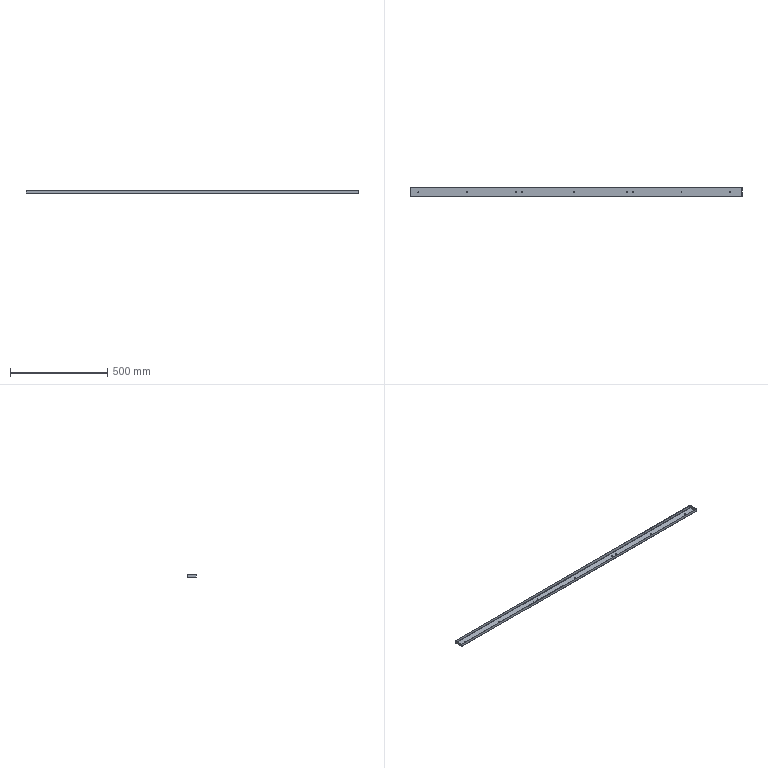Part | STEP file | [01]-3 | 1 solid | 35 faces | box 1704 x 46 x 15 mm | volume 124954 mm3 | cylinder 22 | plane 13 | commonest cylinder face diameters 5 x18 2 x2 4 x2
STEP:
#1=CARTESIAN_POINT('',(1641.,23.,1.));
#2=VERTEX_POINT('',#1);
#3=CARTESIAN_POINT('',(1646.,23.,1.));
#4=VERTEX_POINT('',#3);
#5=CARTESIAN_POINT('',(1643.5,23.,1.));
#6=DIRECTION('',(0.,0.,-1.));
#7=DIRECTION('',(1.,0.,0.));
#8=AXIS2_PLACEMENT_3D('',#5,#6,#7);
#9=CIRCLE('',#8,2.5);
#10=EDGE_CURVE('',#2,#4,#9,.T.);
#11=ORIENTED_EDGE('',*,*,#10,.F.);
#12=CARTESIAN_POINT('',(1641.,23.,0.));
#13=VERTEX_POINT('',#12);
#14=CARTESIAN_POINT('',(1641.,23.,1.));
#15=DIRECTION('',(0.,0.,-1.));
#16=VECTOR('',#15,1000.);
#17=LINE('',#14,#16);
#18=EDGE_CURVE('',#2,#13,#17,.T.);
#19=ORIENTED_EDGE('',*,*,#18,.T.);
#20=CARTESIAN_POINT('',(1646.,23.,0.));
#21=VERTEX_POINT('',#20);
#22=CARTESIAN_POINT('',(1643.5,23.,0.));
#23=DIRECTION('',(0.,0.,1.));
#24=DIRECTION('',(-1.,0.,0.));
#25=AXIS2_PLACEMENT_3D('',#22,#23,#24);
#26=CIRCLE('',#25,2.5);
#27=EDGE_CURVE('',#21,#13,#26,.T.);
#28=ORIENTED_EDGE('',*,*,#27,.F.);
#29=CARTESIAN_POINT('',(1646.,23.,1.));
#30=DIRECTION('',(0.,0.,-1.));
#31=VECTOR('',#30,1000.);
#32=LINE('',#29,#31);
#33=EDGE_CURVE('',#4,#21,#32,.T.);
#34=ORIENTED_EDGE('',*,*,#33,.F.);
#35=EDGE_LOOP('',(#11,#19,#28,#34));
#36=FACE_OUTER_BOUND('',#35,.T.);
#37=CARTESIAN_POINT('',(1643.5,23.,1.));
#38=DIRECTION('',(0.,0.,-1.));
#39=DIRECTION('',(1.,0.,0.));
#40=AXIS2_PLACEMENT_3D('',#37,#38,#39);
#41=CYLINDRICAL_SURFACE('',#40,2.5);
#42=ADVANCED_FACE('',(#36),#41,.F.);
#43=CARTESIAN_POINT('',(1391.,23.,1.));
#44=VERTEX_POINT('',#43);
#45=CARTESIAN_POINT('',(1396.,23.,1.));
#46=VERTEX_POINT('',#45);
#47=CARTESIAN_POINT('',(1393.5,23.,1.));
#48=DIRECTION('',(0.,0.,-1.));
#49=DIRECTION('',(1.,0.,0.));
#50=AXIS2_PLACEMENT_3D('',#47,#48,#49);
#51=CIRCLE('',#50,2.5);
#52=EDGE_CURVE('',#44,#46,#51,.T.);
#53=ORIENTED_EDGE('',*,*,#52,.F.);
#54=CARTESIAN_POINT('',(1391.,23.,0.));
#55=VERTEX_POINT('',#54);
#56=CARTESIAN_POINT('',(1391.,23.,1.));
#57=DIRECTION('',(0.,0.,-1.));
#58=VECTOR('',#57,1000.);
#59=LINE('',#56,#58);
#60=EDGE_CURVE('',#44,#55,#59,.T.);
#61=ORIENTED_EDGE('',*,*,#60,.T.);
#62=CARTESIAN_POINT('',(1396.,23.,0.));
#63=VERTEX_POINT('',#62);
#64=CARTESIAN_POINT('',(1393.5,23.,0.));
#65=DIRECTION('',(0.,0.,1.));
#66=DIRECTION('',(-1.,0.,0.));
#67=AXIS2_PLACEMENT_3D('',#64,#65,#66);
#68=CIRCLE('',#67,2.5);
#69=EDGE_CURVE('',#63,#55,#68,.T.);
#70=ORIENTED_EDGE('',*,*,#69,.F.);
#71=CARTESIAN_POINT('',(1396.,23.,1.));
#72=DIRECTION('',(0.,0.,-1.));
#73=VECTOR('',#72,1000.);
#74=LINE('',#71,#73);
#75=EDGE_CURVE('',#46,#63,#74,.T.);
#76=ORIENTED_EDGE('',*,*,#75,.F.);
#77=EDGE_LOOP('',(#53,#61,#70,#76));
#78=FACE_OUTER_BOUND('',#77,.T.);
#79=CARTESIAN_POINT('',(1393.5,23.,1.));
#80=DIRECTION('',(0.,0.,-1.));
#81=DIRECTION('',(1.,0.,0.));
#82=AXIS2_PLACEMENT_3D('',#79,#80,#81);
#83=CYLINDRICAL_SURFACE('',#82,2.5);
#84=ADVANCED_FACE('',(#78),#83,.F.);
#85=CARTESIAN_POINT('',(1141.,23.,1.));
#86=VERTEX_POINT('',#85);
#87=CARTESIAN_POINT('',(1146.,23.,1.));
#88=VERTEX_POINT('',#87);
#89=CARTESIAN_POINT('',(1143.5,23.,1.));
#90=DIRECTION('',(0.,0.,-1.));
#91=DIRECTION('',(1.,0.,0.));
#92=AXIS2_PLACEMENT_3D('',#89,#90,#91);
#93=CIRCLE('',#92,2.5);
#94=EDGE_CURVE('',#86,#88,#93,.T.);
#95=ORIENTED_EDGE('',*,*,#94,.F.);
#96=CARTESIAN_POINT('',(1141.,23.,0.));
#97=VERTEX_POINT('',#96);
#98=CARTESIAN_POINT('',(1141.,23.,1.));
#99=DIRECTION('',(0.,0.,-1.));
#100=VECTOR('',#99,1000.);
#101=LINE('',#98,#100);
#102=EDGE_CURVE('',#86,#97,#101,.T.);
#103=ORIENTED_EDGE('',*,*,#102,.T.);
#104=CARTESIAN_POINT('',(1146.,23.,0.));
#105=VERTEX_POINT('',#104);
#106=CARTESIAN_POINT('',(1143.5,23.,0.));
#107=DIRECTION('',(0.,0.,1.));
#108=DIRECTION('',(-1.,0.,0.));
#109=AXIS2_PLACEMENT_3D('',#106,#107,#108);
#110=CIRCLE('',#109,2.5);
#111=EDGE_CURVE('',#105,#97,#110,.T.);
#112=ORIENTED_EDGE('',*,*,#111,.F.);
#113=CARTESIAN_POINT('',(1146.,23.,1.));
#114=DIRECTION('',(0.,0.,-1.));
#115=VECTOR('',#114,1000.);
#116=LINE('',#113,#115);
#117=EDGE_CURVE('',#88,#105,#116,.T.);
#118=ORIENTED_EDGE('',*,*,#117,.F.);
#119=EDGE_LOOP('',(#95,#103,#112,#118));
#120=FACE_OUTER_BOUND('',#119,.T.);
#121=CARTESIAN_POINT('',(1143.5,23.,1.));
#122=DIRECTION('',(0.,0.,-1.));
#123=DIRECTION('',(1.,0.,0.));
#124=AXIS2_PLACEMENT_3D('',#121,#122,#123);
#125=CYLINDRICAL_SURFACE('',#124,2.5);
#126=ADVANCED_FACE('',(#120),#125,.F.);
#127=CARTESIAN_POINT('',(1111.,23.,1.));
#128=VERTEX_POINT('',#127);
#129=CARTESIAN_POINT('',(1116.,23.,1.));
#130=VERTEX_POINT('',#129);
#131=CARTESIAN_POINT('',(1113.5,23.,1.));
#132=DIRECTION('',(0.,0.,-1.));
#133=DIRECTION('',(1.,0.,0.));
#134=AXIS2_PLACEMENT_3D('',#131,#132,#133);
#135=CIRCLE('',#134,2.5);
#136=EDGE_CURVE('',#128,#130,#135,.T.);
#137=ORIENTED_EDGE('',*,*,#136,.F.);
#138=CARTESIAN_POINT('',(1111.,23.,0.));
#139=VERTEX_POINT('',#138);
#140=CARTESIAN_POINT('',(1111.,23.,1.));
#141=DIRECTION('',(0.,0.,-1.));
#142=VECTOR('',#141,1000.);
#143=LINE('',#140,#142);
#144=EDGE_CURVE('',#128,#139,#143,.T.);
#145=ORIENTED_EDGE('',*,*,#144,.T.);
#146=CARTESIAN_POINT('',(1116.,23.,0.));
#147=VERTEX_POINT('',#146);
#148=CARTESIAN_POINT('',(1113.5,23.,0.));
#149=DIRECTION('',(0.,0.,1.));
#150=DIRECTION('',(-1.,0.,0.));
#151=AXIS2_PLACEMENT_3D('',#148,#149,#150);
#152=CIRCLE('',#151,2.5);
#153=EDGE_CURVE('',#147,#139,#152,.T.);
#154=ORIENTED_EDGE('',*,*,#153,.F.);
#155=CARTESIAN_POINT('',(1116.,23.,1.));
#156=DIRECTION('',(0.,0.,-1.));
#157=VECTOR('',#156,1000.);
#158=LINE('',#155,#157);
#159=EDGE_CURVE('',#130,#147,#158,.T.);
#160=ORIENTED_EDGE('',*,*,#159,.F.);
#161=EDGE_LOOP('',(#137,#145,#154,#160));
#162=FACE_OUTER_BOUND('',#161,.T.);
#163=CARTESIAN_POINT('',(1113.5,23.,1.));
#164=DIRECTION('',(0.,0.,-1.));
#165=DIRECTION('',(1.,0.,0.));
#166=AXIS2_PLACEMENT_3D('',#163,#164,#165);
#167=CYLINDRICAL_SURFACE('',#166,2.5);
#168=ADVANCED_FACE('',(#162),#167,.F.);
#169=CARTESIAN_POINT('',(841.,23.,1.));
#170=VERTEX_POINT('',#169);
#171=CARTESIAN_POINT('',(846.,23.,1.));
#172=VERTEX_POINT('',#171);
#173=CARTESIAN_POINT('',(843.5,23.,1.));
#174=DIRECTION('',(0.,0.,-1.));
#175=DIRECTION('',(1.,0.,0.));
#176=AXIS2_PLACEMENT_3D('',#173,#174,#175);
#177=CIRCLE('',#176,2.5);
#178=EDGE_CURVE('',#170,#172,#177,.T.);
#179=ORIENTED_EDGE('',*,*,#178,.F.);
#180=CARTESIAN_POINT('',(841.,23.,0.));
#181=VERTEX_POINT('',#180);
#182=CARTESIAN_POINT('',(841.,23.,1.));
#183=DIRECTION('',(0.,0.,-1.));
#184=VECTOR('',#183,1000.);
#185=LINE('',#182,#184);
#186=EDGE_CURVE('',#170,#181,#185,.T.);
#187=ORIENTED_EDGE('',*,*,#186,.T.);
#188=CARTESIAN_POINT('',(846.,23.,0.));
#189=VERTEX_POINT('',#188);
#190=CARTESIAN_POINT('',(843.5,23.,0.));
#191=DIRECTION('',(0.,0.,1.));
#192=DIRECTION('',(-1.,0.,0.));
#193=AXIS2_PLACEMENT_3D('',#190,#191,#192);
#194=CIRCLE('',#193,2.5);
#195=EDGE_CURVE('',#189,#181,#194,.T.);
#196=ORIENTED_EDGE('',*,*,#195,.F.);
#197=CARTESIAN_POINT('',(846.,23.,1.));
#198=DIRECTION('',(0.,0.,-1.));
#199=VECTOR('',#198,1000.);
#200=LINE('',#197,#199);
#201=EDGE_CURVE('',#172,#189,#200,.T.);
#202=ORIENTED_EDGE('',*,*,#201,.F.);
#203=EDGE_LOOP('',(#179,#187,#196,#202));
#204=FACE_OUTER_BOUND('',#203,.T.);
#205=CARTESIAN_POINT('',(843.5,23.,1.));
#206=DIRECTION('',(0.,0.,-1.));
#207=DIRECTION('',(1.,0.,0.));
#208=AXIS2_PLACEMENT_3D('',#205,#206,#207);
#209=CYLINDRICAL_SURFACE('',#208,2.5);
#210=ADVANCED_FACE('',(#204),#209,.F.);
#211=CARTESIAN_POINT('',(571.,23.,1.));
#212=VERTEX_POINT('',#211);
#213=CARTESIAN_POINT('',(576.,23.,1.));
#214=VERTEX_POINT('',#213);
#215=CARTESIAN_POINT('',(573.5,23.,1.));
#216=DIRECTION('',(0.,0.,-1.));
#217=DIRECTION('',(1.,0.,0.));
#218=AXIS2_PLACEMENT_3D('',#215,#216,#217);
#219=CIRCLE('',#218,2.5);
#220=EDGE_CURVE('',#212,#214,#219,.T.);
#221=ORIENTED_EDGE('',*,*,#220,.F.);
#222=CARTESIAN_POINT('',(571.,23.,0.));
#223=VERTEX_POINT('',#222);
#224=CARTESIAN_POINT('',(571.,23.,1.));
#225=DIRECTION('',(0.,0.,-1.));
#226=VECTOR('',#225,1000.);
#227=LINE('',#224,#226);
#228=EDGE_CURVE('',#212,#223,#227,.T.);
#229=ORIENTED_EDGE('',*,*,#228,.T.);
#230=CARTESIAN_POINT('',(576.,23.,0.));
#231=VERTEX_POINT('',#230);
#232=CARTESIAN_POINT('',(573.5,23.,0.));
#233=DIRECTION('',(0.,0.,1.));
#234=DIRECTION('',(-1.,0.,0.));
#235=AXIS2_PLACEMENT_3D('',#232,#233,#234);
#236=CIRCLE('',#235,2.5);
#237=EDGE_CURVE('',#231,#223,#236,.T.);
#238=ORIENTED_EDGE('',*,*,#237,.F.);
#239=CARTESIAN_POINT('',(576.,23.,1.));
#240=DIRECTION('',(0.,0.,-1.));
#241=VECTOR('',#240,1000.);
#242=LINE('',#239,#241);
#243=EDGE_CURVE('',#214,#231,#242,.T.);
#244=ORIENTED_EDGE('',*,*,#243,.F.);
#245=EDGE_LOOP('',(#221,#229,#238,#244));
#246=FACE_OUTER_BOUND('',#245,.T.);
#247=CARTESIAN_POINT('',(573.5,23.,1.));
#248=DIRECTION('',(0.,0.,-1.));
#249=DIRECTION('',(1.,0.,0.));
#250=AXIS2_PLACEMENT_3D('',#247,#248,#249);
#251=CYLINDRICAL_SURFACE('',#250,2.5);
#252=ADVANCED_FACE('',(#246),#251,.F.);
#253=CARTESIAN_POINT('',(541.,23.,1.));
#254=VERTEX_POINT('',#253);
#255=CARTESIAN_POINT('',(546.,23.,1.));
#256=VERTEX_POINT('',#255);
#257=CARTESIAN_POINT('',(543.5,23.,1.));
#258=DIRECTION('',(0.,0.,-1.));
#259=DIRECTION('',(1.,0.,0.));
#260=AXIS2_PLACEMENT_3D('',#257,#258,#259);
#261=CIRCLE('',#260,2.5);
#262=EDGE_CURVE('',#254,#256,#261,.T.);
#263=ORIENTED_EDGE('',*,*,#262,.F.);
#264=CARTESIAN_POINT('',(541.,23.,0.));
#265=VERTEX_POINT('',#264);
#266=CARTESIAN_POINT('',(541.,23.,1.));
#267=DIRECTION('',(0.,0.,-1.));
#268=VECTOR('',#267,1000.);
#269=LINE('',#266,#268);
#270=EDGE_CURVE('',#254,#265,#269,.T.);
#271=ORIENTED_EDGE('',*,*,#270,.T.);
#272=CARTESIAN_POINT('',(546.,23.,0.));
#273=VERTEX_POINT('',#272);
#274=CARTESIAN_POINT('',(543.5,23.,0.));
#275=DIRECTION('',(0.,0.,1.));
#276=DIRECTION('',(-1.,0.,0.));
#277=AXIS2_PLACEMENT_3D('',#274,#275,#276);
#278=CIRCLE('',#277,2.5);
#279=EDGE_CURVE('',#273,#265,#278,.T.);
#280=ORIENTED_EDGE('',*,*,#279,.F.);
#281=CARTESIAN_POINT('',(546.,23.,1.));
#282=DIRECTION('',(0.,0.,-1.));
#283=VECTOR('',#282,1000.);
#284=LINE('',#281,#283);
#285=EDGE_CURVE('',#256,#273,#284,.T.);
#286=ORIENTED_EDGE('',*,*,#285,.F.);
#287=EDGE_LOOP('',(#263,#271,#280,#286));
#288=FACE_OUTER_BOUND('',#287,.T.);
#289=CARTESIAN_POINT('',(543.5,23.,1.));
#290=DIRECTION('',(0.,0.,-1.));
#291=DIRECTION('',(1.,0.,0.));
#292=AXIS2_PLACEMENT_3D('',#289,#290,#291);
#293=CYLINDRICAL_SURFACE('',#292,2.5);
#294=ADVANCED_FACE('',(#288),#293,.F.);
#295=CARTESIAN_POINT('',(291.,23.,1.));
#296=VERTEX_POINT('',#295);
#297=CARTESIAN_POINT('',(296.,23.,1.));
#298=VERTEX_POINT('',#297);
#299=CARTESIAN_POINT('',(293.5,23.,1.));
#300=DIRECTION('',(0.,0.,-1.));
#301=DIRECTION('',(1.,0.,0.));
#302=AXIS2_PLACEMENT_3D('',#299,#300,#301);
#303=CIRCLE('',#302,2.5);
#304=EDGE_CURVE('',#296,#298,#303,.T.);
#305=ORIENTED_EDGE('',*,*,#304,.F.);
#306=CARTESIAN_POINT('',(291.,23.,0.));
#307=VERTEX_POINT('',#306);
#308=CARTESIAN_POINT('',(291.,23.,1.));
#309=DIRECTION('',(0.,0.,-1.));
#310=VECTOR('',#309,1000.);
#311=LINE('',#308,#310);
#312=EDGE_CURVE('',#296,#307,#311,.T.);
#313=ORIENTED_EDGE('',*,*,#312,.T.);
#314=CARTESIAN_POINT('',(296.,23.,0.));
#315=VERTEX_POINT('',#314);
#316=CARTESIAN_POINT('',(293.5,23.,0.));
#317=DIRECTION('',(0.,0.,1.));
#318=DIRECTION('',(-1.,0.,0.));
#319=AXIS2_PLACEMENT_3D('',#316,#317,#318);
#320=CIRCLE('',#319,2.5);
#321=EDGE_CURVE('',#315,#307,#320,.T.);
#322=ORIENTED_EDGE('',*,*,#321,.F.);
#323=CARTESIAN_POINT('',(296.,23.,1.));
#324=DIRECTION('',(0.,0.,-1.));
#325=VECTOR('',#324,1000.);
#326=LINE('',#323,#325);
#327=EDGE_CURVE('',#298,#315,#326,.T.);
#328=ORIENTED_EDGE('',*,*,#327,.F.);
#329=EDGE_LOOP('',(#305,#313,#322,#328));
#330=FACE_OUTER_BOUND('',#329,.T.);
#331=CARTESIAN_POINT('',(293.5,23.,1.));
#332=DIRECTION('',(0.,0.,-1.));
#333=DIRECTION('',(1.,0.,0.));
#334=AXIS2_PLACEMENT_3D('',#331,#332,#333);
#335=CYLINDRICAL_SURFACE('',#334,2.5);
#336=ADVANCED_FACE('',(#330),#335,.F.);
#337=CARTESIAN_POINT('',(41.,23.,1.));
#338=VERTEX_POINT('',#337);
#339=CARTESIAN_POINT('',(46.,23.,1.));
#340=VERTEX_POINT('',#339);
#341=CARTESIAN_POINT('',(43.5,23.,1.));
#342=DIRECTION('',(0.,0.,-1.));
#343=DIRECTION('',(1.,0.,0.));
#344=AXIS2_PLACEMENT_3D('',#341,#342,#343);
#345=CIRCLE('',#344,2.5);
#346=EDGE_CURVE('',#338,#340,#345,.T.);
#347=ORIENTED_EDGE('',*,*,#346,.F.);
#348=CARTESIAN_POINT('',(41.,23.,0.));
#349=VERTEX_POINT('',#348);
#350=CARTESIAN_POINT('',(41.,23.,1.));
#351=DIRECTION('',(0.,0.,-1.));
#352=VECTOR('',#351,1000.);
#353=LINE('',#350,#352);
#354=EDGE_CURVE('',#338,#349,#353,.T.);
#355=ORIENTED_EDGE('',*,*,#354,.T.);
#356=CARTESIAN_POINT('',(46.,23.,0.));
#357=VERTEX_POINT('',#356);
#358=CARTESIAN_POINT('',(43.5,23.,0.));
#359=DIRECTION('',(0.,0.,1.));
#360=DIRECTION('',(-1.,0.,0.));
#361=AXIS2_PLACEMENT_3D('',#358,#359,#360);
#362=CIRCLE('',#361,2.5);
#363=EDGE_CURVE('',#357,#349,#362,.T.);
#364=ORIENTED_EDGE('',*,*,#363,.F.);
#365=CARTESIAN_POINT('',(46.,23.,1.));
#366=DIRECTION('',(0.,0.,-1.));
#367=VECTOR('',#366,1000.);
#368=LINE('',#365,#367);
#369=EDGE_CURVE('',#340,#357,#368,.T.);
#370=ORIENTED_EDGE('',*,*,#369,.F.);
#371=EDGE_LOOP('',(#347,#355,#364,#370));
#372=FACE_OUTER_BOUND('',#371,.T.);
#373=CARTESIAN_POINT('',(43.5,23.,1.));
#374=DIRECTION('',(0.,0.,-1.));
#375=DIRECTION('',(1.,0.,0.));
#376=AXIS2_PLACEMENT_3D('',#373,#374,#375);
#377=CYLINDRICAL_SURFACE('',#376,2.5);
#378=ADVANCED_FACE('',(#372),#377,.F.);
#379=CARTESIAN_POINT('',(1.,45.,2.));
#380=VERTEX_POINT('',#379);
#381=CARTESIAN_POINT('',(1703.,45.,2.));
#382=VERTEX_POINT('',#381);
#383=CARTESIAN_POINT('',(1704.,45.,2.));
#384=DIRECTION('',(1.,0.,0.));
#385=VECTOR('',#384,1000.);
#386=LINE('',#383,#385);
#387=EDGE_CURVE('',#380,#382,#386,.T.);
#388=ORIENTED_EDGE('',*,*,#387,.T.);
#389=CARTESIAN_POINT('',(1703.,45.,14.));
#390=VERTEX_POINT('',#389);
#391=CARTESIAN_POINT('',(1703.,45.,2.));
#392=DIRECTION('',(0.,0.,1.));
#393=VECTOR('',#392,1000.);
#394=LINE('',#391,#393);
#395=EDGE_CURVE('',#382,#390,#394,.T.);
#396=ORIENTED_EDGE('',*,*,#395,.T.);
#397=CARTESIAN_POINT('',(1702.,45.,15.));
#398=VERTEX_POINT('',#397);
#399=CARTESIAN_POINT('',(1704.,45.,13.));
#400=DIRECTION('',(-0.7071,0.,0.7071));
#401=VECTOR('',#400,1000.);
#402=LINE('',#399,#401);
#403=EDGE_CURVE('',#390,#398,#402,.T.);
#404=ORIENTED_EDGE('',*,*,#403,.T.);
#405=CARTESIAN_POINT('',(1.,45.,15.));
#406=VERTEX_POINT('',#405);
#407=CARTESIAN_POINT('',(1702.,45.,15.));
#408=DIRECTION('',(-1.,0.,0.));
#409=VECTOR('',#408,1000.);
#410=LINE('',#407,#409);
#411=EDGE_CURVE('',#398,#406,#410,.T.);
#412=ORIENTED_EDGE('',*,*,#411,.T.);
#413=CARTESIAN_POINT('',(1.,45.,2.));
#414=DIRECTION('',(0.,0.,1.));
#415=VECTOR('',#414,1000.);
#416=LINE('',#413,#415);
#417=EDGE_CURVE('',#380,#406,#416,.T.);
#418=ORIENTED_EDGE('',*,*,#417,.F.);
#419=EDGE_LOOP('',(#388,#396,#404,#412,#418));
#420=FACE_OUTER_BOUND('',#419,.T.);
#421=CARTESIAN_POINT('',(1831.848,45.,1431.971));
#422=DIRECTION('',(0.,-1.,0.));
#423=DIRECTION('',(1.,0.,0.));
#424=AXIS2_PLACEMENT_3D('',#421,#422,#423);
#425=PLANE('',#424);
#426=ADVANCED_FACE('',(#420),#425,.T.);
#427=CARTESIAN_POINT('',(1643.5,23.,1.));
#428=DIRECTION('',(0.,0.,-1.));
#429=DIRECTION('',(1.,0.,0.));
#430=AXIS2_PLACEMENT_3D('',#427,#428,#429);
#431=CIRCLE('',#430,2.5);
#432=EDGE_CURVE('',#4,#2,#431,.T.);
#433=ORIENTED_EDGE('',*,*,#432,.T.);
#434=ORIENTED_EDGE('',*,*,#10,.T.);
#435=EDGE_LOOP('',(#433,#434));
#436=FACE_BOUND('',#435,.T.);
#437=CARTESIAN_POINT('',(1393.5,23.,1.));
#438=DIRECTION('',(0.,0.,-1.));
#439=DIRECTION('',(1.,0.,0.));
#440=AXIS2_PLACEMENT_3D('',#437,#438,#439);
#441=CIRCLE('',#440,2.5);
#442=EDGE_CURVE('',#46,#44,#441,.T.);
#443=ORIENTED_EDGE('',*,*,#442,.T.);
#444=ORIENTED_EDGE('',*,*,#52,.T.);
#445=EDGE_LOOP('',(#443,#444));
#446=FACE_BOUND('',#445,.T.);
#447=CARTESIAN_POINT('',(1143.5,23.,1.));
#448=DIRECTION('',(0.,0.,-1.));
#449=DIRECTION('',(1.,0.,0.));
#450=AXIS2_PLACEMENT_3D('',#447,#448,#449);
#451=CIRCLE('',#450,2.5);
#452=EDGE_CURVE('',#88,#86,#451,.T.);
#453=ORIENTED_EDGE('',*,*,#452,.T.);
#454=ORIENTED_EDGE('',*,*,#94,.T.);
#455=EDGE_LOOP('',(#453,#454));
#456=FACE_BOUND('',#455,.T.);
#457=CARTESIAN_POINT('',(1113.5,23.,1.));
#458=DIRECTION('',(0.,0.,-1.));
#459=DIRECTION('',(1.,0.,0.));
#460=AXIS2_PLACEMENT_3D('',#457,#458,#459);
#461=CIRCLE('',#460,2.5);
#462=EDGE_CURVE('',#130,#128,#461,.T.);
#463=ORIENTED_EDGE('',*,*,#462,.T.);
#464=ORIENTED_EDGE('',*,*,#136,.T.);
#465=EDGE_LOOP('',(#463,#464));
#466=FACE_BOUND('',#465,.T.);
#467=CARTESIAN_POINT('',(843.5,23.,1.));
#468=DIRECTION('',(0.,0.,-1.));
#469=DIRECTION('',(1.,0.,0.));
#470=AXIS2_PLACEMENT_3D('',#467,#468,#469);
#471=CIRCLE('',#470,2.5);
#472=EDGE_CURVE('',#172,#170,#471,.T.);
#473=ORIENTED_EDGE('',*,*,#472,.T.);
#474=ORIENTED_EDGE('',*,*,#178,.T.);
#475=EDGE_LOOP('',(#473,#474));
#476=FACE_BOUND('',#475,.T.);
#477=CARTESIAN_POINT('',(573.5,23.,1.));
#478=DIRECTION('',(0.,0.,-1.));
#479=DIRECTION('',(1.,0.,0.));
#480=AXIS2_PLACEMENT_3D('',#477,#478,#479);
#481=CIRCLE('',#480,2.5);
#482=EDGE_CURVE('',#214,#212,#481,.T.);
#483=ORIENTED_EDGE('',*,*,#482,.T.);
#484=ORIENTED_EDGE('',*,*,#220,.T.);
#485=EDGE_LOOP('',(#483,#484));
#486=FACE_BOUND('',#485,.T.);
#487=CARTESIAN_POINT('',(543.5,23.,1.));
#488=DIRECTION('',(0.,0.,-1.));
#489=DIRECTION('',(1.,0.,0.));
#490=AXIS2_PLACEMENT_3D('',#487,#488,#489);
#491=CIRCLE('',#490,2.5);
#492=EDGE_CURVE('',#256,#254,#491,.T.);
#493=ORIENTED_EDGE('',*,*,#492,.T.);
#494=ORIENTED_EDGE('',*,*,#262,.T.);
#495=EDGE_LOOP('',(#493,#494));
#496=FACE_BOUND('',#495,.T.);
#497=CARTESIAN_POINT('',(293.5,23.,1.));
#498=DIRECTION('',(0.,0.,-1.));
#499=DIRECTION('',(1.,0.,0.));
#500=AXIS2_PLACEMENT_3D('',#497,#498,#499);
#501=CIRCLE('',#500,2.5);
#502=EDGE_CURVE('',#298,#296,#501,.T.);
#503=ORIENTED_EDGE('',*,*,#502,.T.);
#504=ORIENTED_EDGE('',*,*,#304,.T.);
#505=EDGE_LOOP('',(#503,#504));
#506=FACE_BOUND('',#505,.T.);
#507=CARTESIAN_POINT('',(43.5,23.,1.));
#508=DIRECTION('',(0.,0.,-1.));
#509=DIRECTION('',(1.,0.,0.));
#510=AXIS2_PLACEMENT_3D('',#507,#508,#509);
#511=CIRCLE('',#510,2.5);
#512=EDGE_CURVE('',#340,#338,#511,.T.);
#513=ORIENTED_EDGE('',*,*,#512,.T.);
#514=ORIENTED_EDGE('',*,*,#346,.T.);
#515=EDGE_LOOP('',(#513,#514));
#516=FACE_BOUND('',#515,.T.);
#517=CARTESIAN_POINT('',(1.,2.,1.));
#518=VERTEX_POINT('',#517);
#519=CARTESIAN_POINT('',(1703.,2.,1.));
#520=VERTEX_POINT('',#519);
#521=CARTESIAN_POINT('',(1704.,2.,1.));
#522=DIRECTION('',(1.,0.,0.));
#523=VECTOR('',#522,1000.);
#524=LINE('',#521,#523);
#525=EDGE_CURVE('',#518,#520,#524,.T.);
#526=ORIENTED_EDGE('',*,*,#525,.T.);
#527=CARTESIAN_POINT('',(1703.,44.,1.));
#528=VERTEX_POINT('',#527);
#529=CARTESIAN_POINT('',(1703.,2.,1.));
#530=DIRECTION('',(0.,1.,0.));
#531=VECTOR('',#530,1000.);
#532=LINE('',#529,#531);
#533=EDGE_CURVE('',#520,#528,#532,.T.);
#534=ORIENTED_EDGE('',*,*,#533,.T.);
#535=CARTESIAN_POINT('',(1.,44.,1.));
#536=VERTEX_POINT('',#535);
#537=CARTESIAN_POINT('',(0.,44.,1.));
#538=DIRECTION('',(-1.,0.,0.));
#539=VECTOR('',#538,1000.);
#540=LINE('',#537,#539);
#541=EDGE_CURVE('',#528,#536,#540,.T.);
#542=ORIENTED_EDGE('',*,*,#541,.T.);
#543=CARTESIAN_POINT('',(1.,2.,1.));
#544=DIRECTION('',(0.,1.,0.));
#545=VECTOR('',#544,1000.);
#546=LINE('',#543,#545);
#547=EDGE_CURVE('',#518,#536,#546,.T.);
#548=ORIENTED_EDGE('',*,*,#547,.F.);
#549=EDGE_LOOP('',(#526,#534,#542,#548));
#550=FACE_OUTER_BOUND('',#549,.T.);
#551=CARTESIAN_POINT('',(1704.,46.,1.));
#552=DIRECTION('',(0.,0.,1.));
#553=DIRECTION('',(-1.,0.,0.));
#554=AXIS2_PLACEMENT_3D('',#551,#552,#553);
#555=PLANE('',#554);
#556=ADVANCED_FACE('',(#436,#446,#456,#466,#476,#486,#496,#506,#516,#550),#555,.T.);
#557=CARTESIAN_POINT('',(1703.,44.,2.));
#558=DIRECTION('',(1.,0.,0.));
#559=DIRECTION('',(0.,1.,0.));
#560=AXIS2_PLACEMENT_3D('',#557,#558,#559);
#561=CIRCLE('',#560,1.);
#562=EDGE_CURVE('',#528,#382,#561,.T.);
#563=ORIENTED_EDGE('',*,*,#562,.T.);
#564=ORIENTED_EDGE('',*,*,#387,.F.);
#565=CARTESIAN_POINT('',(1.,44.,2.));
#566=DIRECTION('',(1.,0.,0.));
#567=DIRECTION('',(0.,1.,0.));
#568=AXIS2_PLACEMENT_3D('',#565,#566,#567);
#569=CIRCLE('',#568,1.);
#570=EDGE_CURVE('',#536,#380,#569,.T.);
#571=ORIENTED_EDGE('',*,*,#570,.F.);
#572=ORIENTED_EDGE('',*,*,#541,.F.);
#573=EDGE_LOOP('',(#563,#564,#571,#572));
#574=FACE_OUTER_BOUND('',#573,.T.);
#575=CARTESIAN_POINT('',(1831.848,44.,2.));
#576=DIRECTION('',(-1.,0.,0.));
#577=DIRECTION('',(0.,0.,-1.));
#578=AXIS2_PLACEMENT_3D('',#575,#576,#577);
#579=CYLINDRICAL_SURFACE('',#578,1.);
#580=ADVANCED_FACE('',(#574),#579,.F.);
#581=CARTESIAN_POINT('',(1703.,1.,2.));
#582=VERTEX_POINT('',#581);
#583=CARTESIAN_POINT('',(1703.,2.,2.));
#584=DIRECTION('',(1.,0.,0.));
#585=DIRECTION('',(0.,1.,0.));
#586=AXIS2_PLACEMENT_3D('',#583,#584,#585);
#587=CIRCLE('',#586,1.);
#588=EDGE_CURVE('',#582,#520,#587,.T.);
#589=ORIENTED_EDGE('',*,*,#588,.T.);
#590=ORIENTED_EDGE('',*,*,#525,.F.);
#591=CARTESIAN_POINT('',(1.,1.,2.));
#592=VERTEX_POINT('',#591);
#593=CARTESIAN_POINT('',(1.,2.,2.));
#594=DIRECTION('',(1.,0.,0.));
#595=DIRECTION('',(0.,1.,0.));
#596=AXIS2_PLACEMENT_3D('',#593,#594,#595);
#597=CIRCLE('',#596,1.);
#598=EDGE_CURVE('',#592,#518,#597,.T.);
#599=ORIENTED_EDGE('',*,*,#598,.F.);
#600=CARTESIAN_POINT('',(1831.848,1.,2.));
#601=DIRECTION('',(-1.,0.,0.));
#602=VECTOR('',#601,1000.);
#603=LINE('',#600,#602);
#604=EDGE_CURVE('',#582,#592,#603,.T.);
#605=ORIENTED_EDGE('',*,*,#604,.F.);
#606=EDGE_LOOP('',(#589,#590,#599,#605));
#607=FACE_OUTER_BOUND('',#606,.T.);
#608=CARTESIAN_POINT('',(1704.,2.,2.));
#609=DIRECTION('',(1.,0.,0.));
#610=DIRECTION('',(0.,0.,1.));
#611=AXIS2_PLACEMENT_3D('',#608,#609,#610);
#612=CYLINDRICAL_SURFACE('',#611,1.);
#613=ADVANCED_FACE('',(#607),#612,.F.);
#614=CARTESIAN_POINT('',(1703.,1.,15.));
#615=VERTEX_POINT('',#614);
#616=CARTESIAN_POINT('',(1.,1.,15.));
#617=VERTEX_POINT('',#616);
#618=CARTESIAN_POINT('',(1704.,1.,15.));
#619=DIRECTION('',(-1.,0.,0.));
#620=VECTOR('',#619,1000.);
#621=LINE('',#618,#620);
#622=EDGE_CURVE('',#615,#617,#621,.T.);
#623=ORIENTED_EDGE('',*,*,#622,.F.);
#624=CARTESIAN_POINT('',(1703.,1.,15.));
#625=DIRECTION('',(0.,0.,-1.));
#626=VECTOR('',#625,1000.);
#627=LINE('',#624,#626);
#628=EDGE_CURVE('',#615,#582,#627,.T.);
#629=ORIENTED_EDGE('',*,*,#628,.T.);
#630=ORIENTED_EDGE('',*,*,#604,.T.);
#631=CARTESIAN_POINT('',(1.,1.,15.));
#632=DIRECTION('',(0.,0.,-1.));
#633=VECTOR('',#632,1000.);
#634=LINE('',#631,#633);
#635=EDGE_CURVE('',#617,#592,#634,.T.);
#636=ORIENTED_EDGE('',*,*,#635,.F.);
#637=EDGE_LOOP('',(#623,#629,#630,#636));
#638=FACE_OUTER_BOUND('',#637,.T.);
#639=CARTESIAN_POINT('',(1831.848,1.,1431.971));
#640=DIRECTION('',(0.,-1.,0.));
#641=DIRECTION('',(1.,0.,0.));
#642=AXIS2_PLACEMENT_3D('',#639,#640,#641);
#643=PLANE('',#642);
#644=ADVANCED_FACE('',(#638),#643,.F.);
#645=CARTESIAN_POINT('',(1704.,46.,13.));
#646=VERTEX_POINT('',#645);
#647=CARTESIAN_POINT('',(1702.,46.,15.));
#648=VERTEX_POINT('',#647);
#649=CARTESIAN_POINT('',(1704.,46.,13.));
#650=DIRECTION('',(-0.7071,0.,0.7071));
#651=VECTOR('',#650,1000.);
#652=LINE('',#649,#651);
#653=EDGE_CURVE('',#646,#648,#652,.T.);
#654=ORIENTED_EDGE('',*,*,#653,.T.);
#655=CARTESIAN_POINT('',(1702.,45.,15.));
#656=DIRECTION('',(0.,1.,0.));
#657=VECTOR('',#656,1000.);
#658=LINE('',#655,#657);
#659=EDGE_CURVE('',#398,#648,#658,.T.);
#660=ORIENTED_EDGE('',*,*,#659,.F.);
#661=ORIENTED_EDGE('',*,*,#403,.F.);
#662=CARTESIAN_POINT('',(1704.,45.,13.));
#663=VERTEX_POINT('',#662);
#664=CARTESIAN_POINT('',(1704.,45.,13.));
#665=DIRECTION('',(-0.7071,0.,0.7071));
#666=VECTOR('',#665,1000.);
#667=LINE('',#664,#666);
#668=EDGE_CURVE('',#663,#390,#667,.T.);
#669=ORIENTED_EDGE('',*,*,#668,.F.);
#670=CARTESIAN_POINT('',(1704.,45.,13.));
#671=DIRECTION('',(0.,1.,0.));
#672=VECTOR('',#671,1000.);
#673=LINE('',#670,#672);
#674=EDGE_CURVE('',#663,#646,#673,.T.);
#675=ORIENTED_EDGE('',*,*,#674,.T.);
#676=EDGE_LOOP('',(#654,#660,#661,#669,#675));
#677=FACE_OUTER_BOUND('',#676,.T.);
#678=CARTESIAN_POINT('',(1704.,45.,13.));
#679=DIRECTION('',(-0.7071,0.,-0.7071));
#680=DIRECTION('',(0.7071,0.,-0.7071));
#681=AXIS2_PLACEMENT_3D('',#678,#679,#680);
#682=PLANE('',#681);
#683=ADVANCED_FACE('',(#677),#682,.F.);
#684=CARTESIAN_POINT('',(0.,46.,15.));
#685=VERTEX_POINT('',#684);
#686=CARTESIAN_POINT('',(1702.,46.,15.));
#687=DIRECTION('',(-1.,0.,0.));
#688=VECTOR('',#687,1000.);
#689=LINE('',#686,#688);
#690=EDGE_CURVE('',#648,#685,#689,.T.);
#691=ORIENTED_EDGE('',*,*,#690,.T.);
#692=CARTESIAN_POINT('',(0.,0.,15.));
#693=VERTEX_POINT('',#692);
#694=CARTESIAN_POINT('',(0.,45.,15.));
#695=DIRECTION('',(0.,1.,0.));
#696=VECTOR('',#695,1000.);
#697=LINE('',#694,#696);
#698=EDGE_CURVE('',#693,#685,#697,.T.);
#699=ORIENTED_EDGE('',*,*,#698,.F.);
#700=CARTESIAN_POINT('',(1704.,0.,15.));
#701=VERTEX_POINT('',#700);
#702=CARTESIAN_POINT('',(1704.,0.,15.));
#703=DIRECTION('',(-1.,0.,0.));
#704=VECTOR('',#703,1000.);
#705=LINE('',#702,#704);
#706=EDGE_CURVE('',#701,#693,#705,.T.);
#707=ORIENTED_EDGE('',*,*,#706,.F.);
#708=CARTESIAN_POINT('',(1704.,45.,15.));
#709=VERTEX_POINT('',#708);
#710=CARTESIAN_POINT('',(1704.,1.,15.));
#711=DIRECTION('',(0.,-1.,0.));
#712=VECTOR('',#711,1000.);
#713=LINE('',#710,#712);
#714=EDGE_CURVE('',#709,#701,#713,.T.);
#715=ORIENTED_EDGE('',*,*,#714,.F.);
#716=CARTESIAN_POINT('',(1703.,45.,15.));
#717=VERTEX_POINT('',#716);
#718=CARTESIAN_POINT('',(1704.,45.,15.));
#719=DIRECTION('',(-1.,0.,0.));
#720=VECTOR('',#719,1000.);
#721=LINE('',#718,#720);
#722=EDGE_CURVE('',#709,#717,#721,.T.);
#723=ORIENTED_EDGE('',*,*,#722,.T.);
#724=CARTESIAN_POINT('',(1703.,45.,15.));
#725=DIRECTION('',(0.,-1.,0.));
#726=VECTOR('',#725,1000.);
#727=LINE('',#724,#726);
#728=EDGE_CURVE('',#717,#615,#727,.T.);
#729=ORIENTED_EDGE('',*,*,#728,.T.);
#730=ORIENTED_EDGE('',*,*,#622,.T.);
#731=CARTESIAN_POINT('',(1.,45.,15.));
#732=DIRECTION('',(0.,-1.,0.));
#733=VECTOR('',#732,1000.);
#734=LINE('',#731,#733);
#735=EDGE_CURVE('',#406,#617,#734,.T.);
#736=ORIENTED_EDGE('',*,*,#735,.F.);
#737=ORIENTED_EDGE('',*,*,#411,.F.);
#738=ORIENTED_EDGE('',*,*,#659,.T.);
#739=EDGE_LOOP('',(#691,#699,#707,#715,#723,#729,#730,#736,#737,#738));
#740=FACE_OUTER_BOUND('',#739,.T.);
#741=CARTESIAN_POINT('',(1702.,45.,15.));
#742=DIRECTION('',(0.,0.,-1.));
#743=DIRECTION('',(1.,0.,0.));
#744=AXIS2_PLACEMENT_3D('',#741,#742,#743);
#745=PLANE('',#744);
#746=ADVANCED_FACE('',(#740),#745,.F.);
#747=CARTESIAN_POINT('',(0.,0.,2.));
#748=VERTEX_POINT('',#747);
#749=CARTESIAN_POINT('',(0.,0.,1.));
#750=DIRECTION('',(0.,0.,-1.));
#751=VECTOR('',#750,1000.);
#752=LINE('',#749,#751);
#753=EDGE_CURVE('',#693,#748,#752,.T.);
#754=ORIENTED_EDGE('',*,*,#753,.F.);
#755=ORIENTED_EDGE('',*,*,#698,.T.);
#756=CARTESIAN_POINT('',(0.,46.,2.));
#757=VERTEX_POINT('',#756);
#758=CARTESIAN_POINT('',(0.,46.,15.));
#759=DIRECTION('',(0.,0.,-1.));
#760=VECTOR('',#759,1000.);
#761=LINE('',#758,#760);
#762=EDGE_CURVE('',#685,#757,#761,.T.);
#763=ORIENTED_EDGE('',*,*,#762,.T.);
#764=CARTESIAN_POINT('',(0.,44.,0.));
#765=VERTEX_POINT('',#764);
#766=CARTESIAN_POINT('',(0.,44.,2.));
#767=DIRECTION('',(-1.,0.,0.));
#768=DIRECTION('',(0.,1.,0.));
#769=AXIS2_PLACEMENT_3D('',#766,#767,#768);
#770=CIRCLE('',#769,2.);
#771=EDGE_CURVE('',#757,#765,#770,.T.);
#772=ORIENTED_EDGE('',*,*,#771,.T.);
#773=CARTESIAN_POINT('',(0.,2.,0.));
#774=VERTEX_POINT('',#773);
#775=CARTESIAN_POINT('',(0.,46.,0.));
#776=DIRECTION('',(0.,-1.,0.));
#777=VECTOR('',#776,1000.);
#778=LINE('',#775,#777);
#779=EDGE_CURVE('',#765,#774,#778,.T.);
#780=ORIENTED_EDGE('',*,*,#779,.T.);
#781=CARTESIAN_POINT('',(0.,2.,2.));
#782=DIRECTION('',(-1.,0.,0.));
#783=DIRECTION('',(0.,1.,0.));
#784=AXIS2_PLACEMENT_3D('',#781,#782,#783);
#785=CIRCLE('',#784,2.);
#786=EDGE_CURVE('',#774,#748,#785,.T.);
#787=ORIENTED_EDGE('',*,*,#786,.T.);
#788=EDGE_LOOP('',(#754,#755,#763,#772,#780,#787));
#789=FACE_OUTER_BOUND('',#788,.T.);
#790=CARTESIAN_POINT('',(0.,45.,15.));
#791=DIRECTION('',(1.,0.,0.));
#792=DIRECTION('',(0.,1.,0.));
#793=AXIS2_PLACEMENT_3D('',#790,#791,#792);
#794=PLANE('',#793);
#795=ADVANCED_FACE('',(#789),#794,.F.);
#796=CARTESIAN_POINT('',(1704.,45.,2.));
#797=DIRECTION('',(0.,0.,1.));
#798=VECTOR('',#797,1000.);
#799=LINE('',#796,#798);
#800=EDGE_CURVE('',#663,#709,#799,.T.);
#801=ORIENTED_EDGE('',*,*,#800,.T.);
#802=ORIENTED_EDGE('',*,*,#714,.T.);
#803=CARTESIAN_POINT('',(1704.,0.,2.));
#804=VERTEX_POINT('',#803);
#805=CARTESIAN_POINT('',(1704.,0.,0.));
#806=DIRECTION('',(0.,0.,1.));
#807=VECTOR('',#806,1000.);
#808=LINE('',#805,#807);
#809=EDGE_CURVE('',#804,#701,#808,.T.);
#810=ORIENTED_EDGE('',*,*,#809,.F.);
#811=CARTESIAN_POINT('',(1704.,2.,0.));
#812=VERTEX_POINT('',#811);
#813=CARTESIAN_POINT('',(1704.,2.,2.));
#814=DIRECTION('',(1.,0.,0.));
#815=DIRECTION('',(0.,-1.,0.));
#816=AXIS2_PLACEMENT_3D('',#813,#814,#815);
#817=CIRCLE('',#816,2.);
#818=EDGE_CURVE('',#804,#812,#817,.T.);
#819=ORIENTED_EDGE('',*,*,#818,.T.);
#820=CARTESIAN_POINT('',(1704.,44.,0.));
#821=VERTEX_POINT('',#820);
#822=CARTESIAN_POINT('',(1704.,46.,0.));
#823=DIRECTION('',(0.,-1.,0.));
#824=VECTOR('',#823,1000.);
#825=LINE('',#822,#824);
#826=EDGE_CURVE('',#821,#812,#825,.T.);
#827=ORIENTED_EDGE('',*,*,#826,.F.);
#828=CARTESIAN_POINT('',(1704.,46.,2.));
#829=VERTEX_POINT('',#828);
#830=CARTESIAN_POINT('',(1704.,44.,2.));
#831=DIRECTION('',(1.,0.,0.));
#832=DIRECTION('',(0.,-1.,0.));
#833=AXIS2_PLACEMENT_3D('',#830,#831,#832);
#834=CIRCLE('',#833,2.);
#835=EDGE_CURVE('',#821,#829,#834,.T.);
#836=ORIENTED_EDGE('',*,*,#835,.T.);
#837=CARTESIAN_POINT('',(1704.,46.,1.));
#838=DIRECTION('',(0.,0.,1.));
#839=VECTOR('',#838,1000.);
#840=LINE('',#837,#839);
#841=EDGE_CURVE('',#829,#646,#840,.T.);
#842=ORIENTED_EDGE('',*,*,#841,.T.);
#843=ORIENTED_EDGE('',*,*,#674,.F.);
#844=EDGE_LOOP('',(#801,#802,#810,#819,#827,#836,#842,#843));
#845=FACE_OUTER_BOUND('',#844,.T.);
#846=CARTESIAN_POINT('',(1704.,45.,1.));
#847=DIRECTION('',(-1.,0.,0.));
#848=DIRECTION('',(0.,-1.,0.));
#849=AXIS2_PLACEMENT_3D('',#846,#847,#848);
#850=PLANE('',#849);
#851=ADVANCED_FACE('',(#845),#850,.F.);
#852=ORIENTED_EDGE('',*,*,#841,.F.);
#853=CARTESIAN_POINT('',(0.,46.,2.));
#854=DIRECTION('',(-1.,0.,0.));
#855=VECTOR('',#854,1000.);
#856=LINE('',#853,#855);
#857=EDGE_CURVE('',#829,#757,#856,.T.);
#858=ORIENTED_EDGE('',*,*,#857,.T.);
#859=ORIENTED_EDGE('',*,*,#762,.F.);
#860=ORIENTED_EDGE('',*,*,#690,.F.);
#861=ORIENTED_EDGE('',*,*,#653,.F.);
#862=EDGE_LOOP('',(#852,#858,#859,#860,#861));
#863=FACE_OUTER_BOUND('',#862,.T.);
#864=CARTESIAN_POINT('',(1831.848,46.,1431.971));
#865=DIRECTION('',(0.,-1.,0.));
#866=DIRECTION('',(1.,0.,0.));
#867=AXIS2_PLACEMENT_3D('',#864,#865,#866);
#868=PLANE('',#867);
#869=ADVANCED_FACE('',(#863),#868,.F.);
#870=ORIENTED_EDGE('',*,*,#27,.T.);
#871=CARTESIAN_POINT('',(1643.5,23.,0.));
#872=DIRECTION('',(0.,0.,1.));
#873=DIRECTION('',(-1.,0.,0.));
#874=AXIS2_PLACEMENT_3D('',#871,#872,#873);
#875=CIRCLE('',#874,2.5);
#876=EDGE_CURVE('',#13,#21,#875,.T.);
#877=ORIENTED_EDGE('',*,*,#876,.T.);
#878=EDGE_LOOP('',(#870,#877));
#879=FACE_BOUND('',#878,.T.);
#880=ORIENTED_EDGE('',*,*,#69,.T.);
#881=CARTESIAN_POINT('',(1393.5,23.,0.));
#882=DIRECTION('',(0.,0.,1.));
#883=DIRECTION('',(-1.,0.,0.));
#884=AXIS2_PLACEMENT_3D('',#881,#882,#883);
#885=CIRCLE('',#884,2.5);
#886=EDGE_CURVE('',#55,#63,#885,.T.);
#887=ORIENTED_EDGE('',*,*,#886,.T.);
#888=EDGE_LOOP('',(#880,#887));
#889=FACE_BOUND('',#888,.T.);
#890=ORIENTED_EDGE('',*,*,#111,.T.);
#891=CARTESIAN_POINT('',(1143.5,23.,0.));
#892=DIRECTION('',(0.,0.,1.));
#893=DIRECTION('',(-1.,0.,0.));
#894=AXIS2_PLACEMENT_3D('',#891,#892,#893);
#895=CIRCLE('',#894,2.5);
#896=EDGE_CURVE('',#97,#105,#895,.T.);
#897=ORIENTED_EDGE('',*,*,#896,.T.);
#898=EDGE_LOOP('',(#890,#897));
#899=FACE_BOUND('',#898,.T.);
#900=ORIENTED_EDGE('',*,*,#153,.T.);
#901=CARTESIAN_POINT('',(1113.5,23.,0.));
#902=DIRECTION('',(0.,0.,1.));
#903=DIRECTION('',(-1.,0.,0.));
#904=AXIS2_PLACEMENT_3D('',#901,#902,#903);
#905=CIRCLE('',#904,2.5);
#906=EDGE_CURVE('',#139,#147,#905,.T.);
#907=ORIENTED_EDGE('',*,*,#906,.T.);
#908=EDGE_LOOP('',(#900,#907));
#909=FACE_BOUND('',#908,.T.);
#910=ORIENTED_EDGE('',*,*,#195,.T.);
#911=CARTESIAN_POINT('',(843.5,23.,0.));
#912=DIRECTION('',(0.,0.,1.));
#913=DIRECTION('',(-1.,0.,0.));
#914=AXIS2_PLACEMENT_3D('',#911,#912,#913);
#915=CIRCLE('',#914,2.5);
#916=EDGE_CURVE('',#181,#189,#915,.T.);
#917=ORIENTED_EDGE('',*,*,#916,.T.);
#918=EDGE_LOOP('',(#910,#917));
#919=FACE_BOUND('',#918,.T.);
#920=ORIENTED_EDGE('',*,*,#237,.T.);
#921=CARTESIAN_POINT('',(573.5,23.,0.));
#922=DIRECTION('',(0.,0.,1.));
#923=DIRECTION('',(-1.,0.,0.));
#924=AXIS2_PLACEMENT_3D('',#921,#922,#923);
#925=CIRCLE('',#924,2.5);
#926=EDGE_CURVE('',#223,#231,#925,.T.);
#927=ORIENTED_EDGE('',*,*,#926,.T.);
#928=EDGE_LOOP('',(#920,#927));
#929=FACE_BOUND('',#928,.T.);
#930=ORIENTED_EDGE('',*,*,#279,.T.);
#931=CARTESIAN_POINT('',(543.5,23.,0.));
#932=DIRECTION('',(0.,0.,1.));
#933=DIRECTION('',(-1.,0.,0.));
#934=AXIS2_PLACEMENT_3D('',#931,#932,#933);
#935=CIRCLE('',#934,2.5);
#936=EDGE_CURVE('',#265,#273,#935,.T.);
#937=ORIENTED_EDGE('',*,*,#936,.T.);
#938=EDGE_LOOP('',(#930,#937));
#939=FACE_BOUND('',#938,.T.);
#940=ORIENTED_EDGE('',*,*,#321,.T.);
#941=CARTESIAN_POINT('',(293.5,23.,0.));
#942=DIRECTION('',(0.,0.,1.));
#943=DIRECTION('',(-1.,0.,0.));
#944=AXIS2_PLACEMENT_3D('',#941,#942,#943);
#945=CIRCLE('',#944,2.5);
#946=EDGE_CURVE('',#307,#315,#945,.T.);
#947=ORIENTED_EDGE('',*,*,#946,.T.);
#948=EDGE_LOOP('',(#940,#947));
#949=FACE_BOUND('',#948,.T.);
#950=ORIENTED_EDGE('',*,*,#363,.T.);
#951=CARTESIAN_POINT('',(43.5,23.,0.));
#952=DIRECTION('',(0.,0.,1.));
#953=DIRECTION('',(-1.,0.,0.));
#954=AXIS2_PLACEMENT_3D('',#951,#952,#953);
#955=CIRCLE('',#954,2.5);
#956=EDGE_CURVE('',#349,#357,#955,.T.);
#957=ORIENTED_EDGE('',*,*,#956,.T.);
#958=EDGE_LOOP('',(#950,#957));
#959=FACE_BOUND('',#958,.T.);
#960=ORIENTED_EDGE('',*,*,#826,.T.);
#961=CARTESIAN_POINT('',(0.,2.,0.));
#962=DIRECTION('',(-1.,0.,0.));
#963=VECTOR('',#962,1000.);
#964=LINE('',#961,#963);
#965=EDGE_CURVE('',#812,#774,#964,.T.);
#966=ORIENTED_EDGE('',*,*,#965,.T.);
#967=ORIENTED_EDGE('',*,*,#779,.F.);
#968=CARTESIAN_POINT('',(1704.,44.,0.));
#969=DIRECTION('',(1.,0.,0.));
#970=VECTOR('',#969,1000.);
#971=LINE('',#968,#970);
#972=EDGE_CURVE('',#765,#821,#971,.T.);
#973=ORIENTED_EDGE('',*,*,#972,.T.);
#974=EDGE_LOOP('',(#960,#966,#967,#973));
#975=FACE_OUTER_BOUND('',#974,.T.);
#976=CARTESIAN_POINT('',(0.,46.,0.));
#977=DIRECTION('',(0.,0.,-1.));
#978=DIRECTION('',(1.,0.,0.));
#979=AXIS2_PLACEMENT_3D('',#976,#977,#978);
#980=PLANE('',#979);
#981=ADVANCED_FACE('',(#879,#889,#899,#909,#919,#929,#939,#949,#959,#975),#980,.T.);
#982=ORIENTED_EDGE('',*,*,#753,.T.);
#983=CARTESIAN_POINT('',(1831.848,0.,2.));
#984=DIRECTION('',(1.,0.,0.));
#985=VECTOR('',#984,1000.);
#986=LINE('',#983,#985);
#987=EDGE_CURVE('',#748,#804,#986,.T.);
#988=ORIENTED_EDGE('',*,*,#987,.T.);
#989=ORIENTED_EDGE('',*,*,#809,.T.);
#990=ORIENTED_EDGE('',*,*,#706,.T.);
#991=EDGE_LOOP('',(#982,#988,#989,#990));
#992=FACE_OUTER_BOUND('',#991,.T.);
#993=CARTESIAN_POINT('',(1831.848,0.,1431.971));
#994=DIRECTION('',(0.,-1.,0.));
#995=DIRECTION('',(1.,0.,0.));
#996=AXIS2_PLACEMENT_3D('',#993,#994,#995);
#997=PLANE('',#996);
#998=ADVANCED_FACE('',(#992),#997,.T.);
#999=ORIENTED_EDGE('',*,*,#771,.F.);
#1000=ORIENTED_EDGE('',*,*,#857,.F.);
#1001=ORIENTED_EDGE('',*,*,#835,.F.);
#1002=ORIENTED_EDGE('',*,*,#972,.F.);
#1003=EDGE_LOOP('',(#999,#1000,#1001,#1002));
#1004=FACE_OUTER_BOUND('',#1003,.T.);
#1005=CARTESIAN_POINT('',(0.,44.,2.));
#1006=DIRECTION('',(-1.,0.,0.));
#1007=DIRECTION('',(0.,0.,-1.));
#1008=AXIS2_PLACEMENT_3D('',#1005,#1006,#1007);
#1009=CYLINDRICAL_SURFACE('',#1008,2.);
#1010=ADVANCED_FACE('',(#1004),#1009,.T.);
#1011=ORIENTED_EDGE('',*,*,#786,.F.);
#1012=ORIENTED_EDGE('',*,*,#965,.F.);
#1013=ORIENTED_EDGE('',*,*,#818,.F.);
#1014=ORIENTED_EDGE('',*,*,#987,.F.);
#1015=EDGE_LOOP('',(#1011,#1012,#1013,#1014));
#1016=FACE_OUTER_BOUND('',#1015,.T.);
#1017=CARTESIAN_POINT('',(1831.848,2.,2.));
#1018=DIRECTION('',(1.,0.,0.));
#1019=DIRECTION('',(0.,0.,1.));
#1020=AXIS2_PLACEMENT_3D('',#1017,#1018,#1019);
#1021=CYLINDRICAL_SURFACE('',#1020,2.);
#1022=ADVANCED_FACE('',(#1016),#1021,.T.);
#1023=ORIENTED_EDGE('',*,*,#354,.F.);
#1024=ORIENTED_EDGE('',*,*,#512,.F.);
#1025=ORIENTED_EDGE('',*,*,#369,.T.);
#1026=ORIENTED_EDGE('',*,*,#956,.F.);
#1027=EDGE_LOOP('',(#1023,#1024,#1025,#1026));
#1028=FACE_OUTER_BOUND('',#1027,.T.);
#1029=CARTESIAN_POINT('',(43.5,23.,1.));
#1030=DIRECTION('',(0.,0.,-1.));
#1031=DIRECTION('',(1.,0.,0.));
#1032=AXIS2_PLACEMENT_3D('',#1029,#1030,#1031);
#1033=CYLINDRICAL_SURFACE('',#1032,2.5);
#1034=ADVANCED_FACE('',(#1028),#1033,.F.);
#1035=ORIENTED_EDGE('',*,*,#312,.F.);
#1036=ORIENTED_EDGE('',*,*,#502,.F.);
#1037=ORIENTED_EDGE('',*,*,#327,.T.);
#1038=ORIENTED_EDGE('',*,*,#946,.F.);
#1039=EDGE_LOOP('',(#1035,#1036,#1037,#1038));
#1040=FACE_OUTER_BOUND('',#1039,.T.);
#1041=CARTESIAN_POINT('',(293.5,23.,1.));
#1042=DIRECTION('',(0.,0.,-1.));
#1043=DIRECTION('',(1.,0.,0.));
#1044=AXIS2_PLACEMENT_3D('',#1041,#1042,#1043);
#1045=CYLINDRICAL_SURFACE('',#1044,2.5);
#1046=ADVANCED_FACE('',(#1040),#1045,.F.);
#1047=ORIENTED_EDGE('',*,*,#270,.F.);
#1048=ORIENTED_EDGE('',*,*,#492,.F.);
#1049=ORIENTED_EDGE('',*,*,#285,.T.);
#1050=ORIENTED_EDGE('',*,*,#936,.F.);
#1051=EDGE_LOOP('',(#1047,#1048,#1049,#1050));
#1052=FACE_OUTER_BOUND('',#1051,.T.);
#1053=CARTESIAN_POINT('',(543.5,23.,1.));
#1054=DIRECTION('',(0.,0.,-1.));
#1055=DIRECTION('',(1.,0.,0.));
#1056=AXIS2_PLACEMENT_3D('',#1053,#1054,#1055);
#1057=CYLINDRICAL_SURFACE('',#1056,2.5);
#1058=ADVANCED_FACE('',(#1052),#1057,.F.);
#1059=ORIENTED_EDGE('',*,*,#228,.F.);
#1060=ORIENTED_EDGE('',*,*,#482,.F.);
#1061=ORIENTED_EDGE('',*,*,#243,.T.);
#1062=ORIENTED_EDGE('',*,*,#926,.F.);
#1063=EDGE_LOOP('',(#1059,#1060,#1061,#1062));
#1064=FACE_OUTER_BOUND('',#1063,.T.);
#1065=CARTESIAN_POINT('',(573.5,23.,1.));
#1066=DIRECTION('',(0.,0.,-1.));
#1067=DIRECTION('',(1.,0.,0.));
#1068=AXIS2_PLACEMENT_3D('',#1065,#1066,#1067);
#1069=CYLINDRICAL_SURFACE('',#1068,2.5);
#1070=ADVANCED_FACE('',(#1064),#1069,.F.);
#1071=ORIENTED_EDGE('',*,*,#186,.F.);
#1072=ORIENTED_EDGE('',*,*,#472,.F.);
#1073=ORIENTED_EDGE('',*,*,#201,.T.);
#1074=ORIENTED_EDGE('',*,*,#916,.F.);
#1075=EDGE_LOOP('',(#1071,#1072,#1073,#1074));
#1076=FACE_OUTER_BOUND('',#1075,.T.);
#1077=CARTESIAN_POINT('',(843.5,23.,1.));
#1078=DIRECTION('',(0.,0.,-1.));
#1079=DIRECTION('',(1.,0.,0.));
#1080=AXIS2_PLACEMENT_3D('',#1077,#1078,#1079);
#1081=CYLINDRICAL_SURFACE('',#1080,2.5);
#1082=ADVANCED_FACE('',(#1076),#1081,.F.);
#1083=ORIENTED_EDGE('',*,*,#144,.F.);
#1084=ORIENTED_EDGE('',*,*,#462,.F.);
#1085=ORIENTED_EDGE('',*,*,#159,.T.);
#1086=ORIENTED_EDGE('',*,*,#906,.F.);
#1087=EDGE_LOOP('',(#1083,#1084,#1085,#1086));
#1088=FACE_OUTER_BOUND('',#1087,.T.);
#1089=CARTESIAN_POINT('',(1113.5,23.,1.));
#1090=DIRECTION('',(0.,0.,-1.));
#1091=DIRECTION('',(1.,0.,0.));
#1092=AXIS2_PLACEMENT_3D('',#1089,#1090,#1091);
#1093=CYLINDRICAL_SURFACE('',#1092,2.5);
#1094=ADVANCED_FACE('',(#1088),#1093,.F.);
#1095=ORIENTED_EDGE('',*,*,#102,.F.);
#1096=ORIENTED_EDGE('',*,*,#452,.F.);
#1097=ORIENTED_EDGE('',*,*,#117,.T.);
#1098=ORIENTED_EDGE('',*,*,#896,.F.);
#1099=EDGE_LOOP('',(#1095,#1096,#1097,#1098));
#1100=FACE_OUTER_BOUND('',#1099,.T.);
#1101=CARTESIAN_POINT('',(1143.5,23.,1.));
#1102=DIRECTION('',(0.,0.,-1.));
#1103=DIRECTION('',(1.,0.,0.));
#1104=AXIS2_PLACEMENT_3D('',#1101,#1102,#1103);
#1105=CYLINDRICAL_SURFACE('',#1104,2.5);
#1106=ADVANCED_FACE('',(#1100),#1105,.F.);
#1107=ORIENTED_EDGE('',*,*,#60,.F.);
#1108=ORIENTED_EDGE('',*,*,#442,.F.);
#1109=ORIENTED_EDGE('',*,*,#75,.T.);
#1110=ORIENTED_EDGE('',*,*,#886,.F.);
#1111=EDGE_LOOP('',(#1107,#1108,#1109,#1110));
#1112=FACE_OUTER_BOUND('',#1111,.T.);
#1113=CARTESIAN_POINT('',(1393.5,23.,1.));
#1114=DIRECTION('',(0.,0.,-1.));
#1115=DIRECTION('',(1.,0.,0.));
#1116=AXIS2_PLACEMENT_3D('',#1113,#1114,#1115);
#1117=CYLINDRICAL_SURFACE('',#1116,2.5);
#1118=ADVANCED_FACE('',(#1112),#1117,.F.);
#1119=ORIENTED_EDGE('',*,*,#18,.F.);
#1120=ORIENTED_EDGE('',*,*,#432,.F.);
#1121=ORIENTED_EDGE('',*,*,#33,.T.);
#1122=ORIENTED_EDGE('',*,*,#876,.F.);
#1123=EDGE_LOOP('',(#1119,#1120,#1121,#1122));
#1124=FACE_OUTER_BOUND('',#1123,.T.);
#1125=CARTESIAN_POINT('',(1643.5,23.,1.));
#1126=DIRECTION('',(0.,0.,-1.));
#1127=DIRECTION('',(1.,0.,0.));
#1128=AXIS2_PLACEMENT_3D('',#1125,#1126,#1127);
#1129=CYLINDRICAL_SURFACE('',#1128,2.5);
#1130=ADVANCED_FACE('',(#1124),#1129,.F.);
#1131=ORIENTED_EDGE('',*,*,#417,.T.);
#1132=ORIENTED_EDGE('',*,*,#735,.T.);
#1133=ORIENTED_EDGE('',*,*,#635,.T.);
#1134=ORIENTED_EDGE('',*,*,#598,.T.);
#1135=ORIENTED_EDGE('',*,*,#547,.T.);
#1136=ORIENTED_EDGE('',*,*,#570,.T.);
#1137=EDGE_LOOP('',(#1131,#1132,#1133,#1134,#1135,#1136));
#1138=FACE_OUTER_BOUND('',#1137,.T.);
#1139=CARTESIAN_POINT('',(1.,2.,2.));
#1140=DIRECTION('',(1.,0.,0.));
#1141=DIRECTION('',(0.,1.,0.));
#1142=AXIS2_PLACEMENT_3D('',#1139,#1140,#1141);
#1143=PLANE('',#1142);
#1144=ADVANCED_FACE('',(#1138),#1143,.T.);
#1145=ORIENTED_EDGE('',*,*,#800,.F.);
#1146=ORIENTED_EDGE('',*,*,#668,.T.);
#1147=CARTESIAN_POINT('',(1703.,45.,2.));
#1148=DIRECTION('',(0.,0.,1.));
#1149=VECTOR('',#1148,1000.);
#1150=LINE('',#1147,#1149);
#1151=EDGE_CURVE('',#390,#717,#1150,.T.);
#1152=ORIENTED_EDGE('',*,*,#1151,.T.);
#1153=ORIENTED_EDGE('',*,*,#722,.F.);
#1154=EDGE_LOOP('',(#1145,#1146,#1152,#1153));
#1155=FACE_OUTER_BOUND('',#1154,.T.);
#1156=CARTESIAN_POINT('',(1704.,45.,2.));
#1157=DIRECTION('',(0.,-1.,0.));
#1158=DIRECTION('',(0.,0.,-1.));
#1159=AXIS2_PLACEMENT_3D('',#1156,#1157,#1158);
#1160=PLANE('',#1159);
#1161=ADVANCED_FACE('',(#1155),#1160,.F.);
#1162=ORIENTED_EDGE('',*,*,#395,.F.);
#1163=ORIENTED_EDGE('',*,*,#562,.F.);
#1164=ORIENTED_EDGE('',*,*,#533,.F.);
#1165=ORIENTED_EDGE('',*,*,#588,.F.);
#1166=ORIENTED_EDGE('',*,*,#628,.F.);
#1167=ORIENTED_EDGE('',*,*,#728,.F.);
#1168=ORIENTED_EDGE('',*,*,#1151,.F.);
#1169=EDGE_LOOP('',(#1162,#1163,#1164,#1165,#1166,#1167,#1168));
#1170=FACE_OUTER_BOUND('',#1169,.T.);
#1171=CARTESIAN_POINT('',(1703.,2.,2.));
#1172=DIRECTION('',(1.,0.,0.));
#1173=DIRECTION('',(0.,1.,0.));
#1174=AXIS2_PLACEMENT_3D('',#1171,#1172,#1173);
#1175=PLANE('',#1174);
#1176=ADVANCED_FACE('',(#1170),#1175,.F.);
#1177=CLOSED_SHELL('',(#42,#84,#126,#168,#210,#252,#294,#336,#378,#426,#556,#580,#613,#644,#683,#746,#795,#851,#869,#981,#998,#1010,#1022,#1034,#1046,#1058,#1070,#1082,#1094,#1106,#1118,#1130,#1144,#1161,#1176));
#1178=MANIFOLD_SOLID_BREP('',#1177);
#1179=CARTESIAN_POINT('',(0.,0.,0.));
#1180=DIRECTION('',(0.,0.,1.));
#1181=DIRECTION('',(1.,0.,0.));
#1182=AXIS2_PLACEMENT_3D('',#1179,#1180,#1181);
#1183=(LENGTH_UNIT()NAMED_UNIT(*)SI_UNIT(.MILLI.,.METRE.));
#1184=UNCERTAINTY_MEASURE_WITH_UNIT(LENGTH_MEASURE(0.00001),#1183,'','');
#1185=(NAMED_UNIT(*)PLANE_ANGLE_UNIT()SI_UNIT($,.RADIAN.));
#1186=(NAMED_UNIT(*)SI_UNIT($,.STERADIAN.)SOLID_ANGLE_UNIT());
#1187=(GEOMETRIC_REPRESENTATION_CONTEXT(3)GLOBAL_UNCERTAINTY_ASSIGNED_CONTEXT((#1184))GLOBAL_UNIT_ASSIGNED_CONTEXT((#1183,#1185,#1186))REPRESENTATION_CONTEXT('',''));
#1188=ADVANCED_BREP_SHAPE_REPRESENTATION('',(#1178,#1182),#1187);